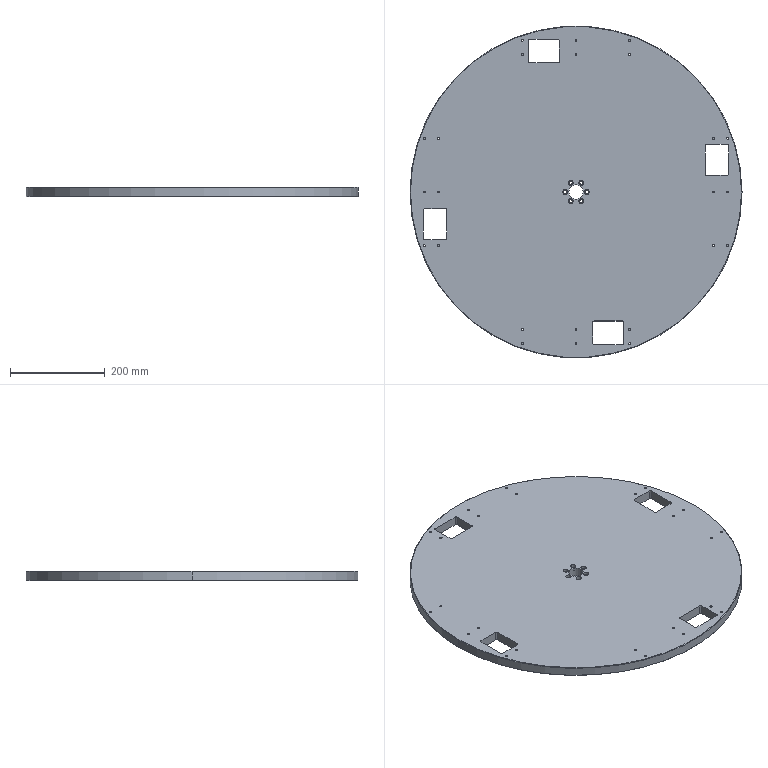Part | STEP file | PN_0009 | 1 solid | 128 faces | box 700 x 700 x 20 mm | volume 7409055 mm3 | cylinder 92 | plane 32 | cone 4 | commonest cylinder face diameters 4.2 x32 5 x16 6 x16 6.6 x12 11 x12 30 x2